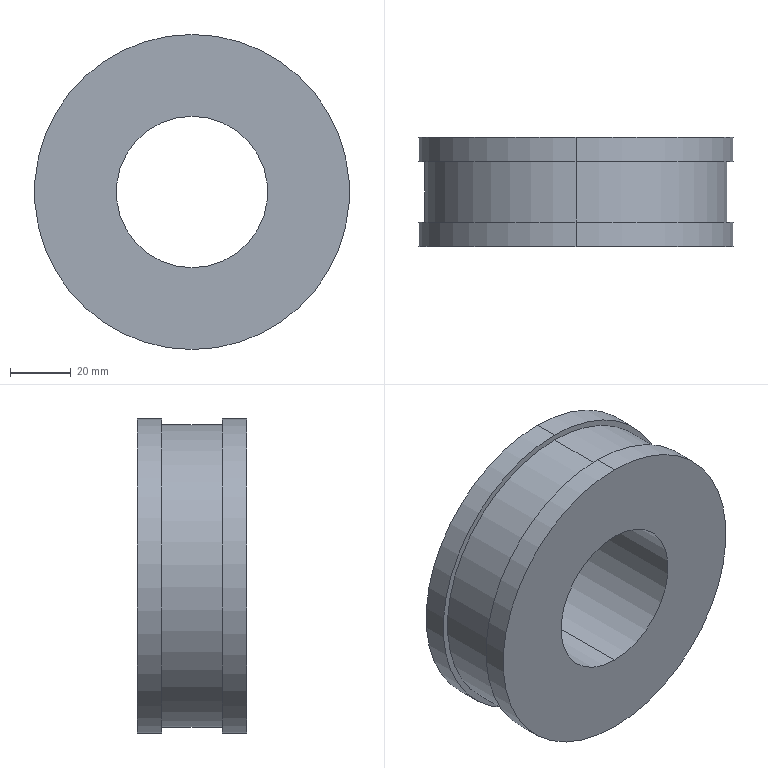Part | SolidWorks | features ICE 3, Extrusion 1 | 1 solid | 12 faces | box 104 x 36 x 104 mm | volume 222312 mm3 | cylinder 8 | plane 4 | commonest cylinder face diameters 104 x4 50 x2 100 x2
STEP:
#1=CARTESIAN_POINT('',(0.,28.,25.));
#2=VERTEX_POINT('',#1);
#3=CARTESIAN_POINT('',(0.,28.,-25.));
#4=VERTEX_POINT('',#3);
#5=CARTESIAN_POINT('',(0.,28.,0.));
#6=DIRECTION('',(0.,-1.,0.));
#7=DIRECTION('',(0.,0.,-1.));
#8=AXIS2_PLACEMENT_3D('',#5,#6,#7);
#9=CIRCLE('',#8,25.);
#10=EDGE_CURVE('',#2,#4,#9,.T.);
#11=ORIENTED_EDGE('',*,*,#10,.F.);
#12=CARTESIAN_POINT('',(0.,-8.,25.));
#13=VERTEX_POINT('',#12);
#14=CARTESIAN_POINT('',(0.,28.,25.));
#15=DIRECTION('',(0.,-1.,0.));
#16=VECTOR('',#15,1000.);
#17=LINE('',#14,#16);
#18=EDGE_CURVE('',#2,#13,#17,.T.);
#19=ORIENTED_EDGE('',*,*,#18,.T.);
#20=CARTESIAN_POINT('',(0.,-8.,-25.));
#21=VERTEX_POINT('',#20);
#22=CARTESIAN_POINT('',(0.,-8.,0.));
#23=DIRECTION('',(0.,-1.,0.));
#24=DIRECTION('',(0.,0.,-1.));
#25=AXIS2_PLACEMENT_3D('',#22,#23,#24);
#26=CIRCLE('',#25,25.);
#27=EDGE_CURVE('',#13,#21,#26,.T.);
#28=ORIENTED_EDGE('',*,*,#27,.T.);
#29=CARTESIAN_POINT('',(0.,28.,-25.));
#30=DIRECTION('',(0.,-1.,0.));
#31=VECTOR('',#30,1000.);
#32=LINE('',#29,#31);
#33=EDGE_CURVE('',#4,#21,#32,.T.);
#34=ORIENTED_EDGE('',*,*,#33,.F.);
#35=EDGE_LOOP('',(#11,#19,#28,#34));
#36=FACE_OUTER_BOUND('',#35,.T.);
#37=CARTESIAN_POINT('',(0.,28.,0.));
#38=DIRECTION('',(0.,-1.,0.));
#39=DIRECTION('',(0.,0.,-1.));
#40=AXIS2_PLACEMENT_3D('',#37,#38,#39);
#41=CYLINDRICAL_SURFACE('',#40,25.);
#42=ADVANCED_FACE('',(#36),#41,.F.);
#43=CARTESIAN_POINT('',(0.,-8.,-52.));
#44=VERTEX_POINT('',#43);
#45=CARTESIAN_POINT('',(0.,-8.,52.));
#46=VERTEX_POINT('',#45);
#47=CARTESIAN_POINT('',(0.,-8.,0.));
#48=DIRECTION('',(0.,-1.,0.));
#49=DIRECTION('',(0.,0.,-1.));
#50=AXIS2_PLACEMENT_3D('',#47,#48,#49);
#51=CIRCLE('',#50,52.);
#52=EDGE_CURVE('',#44,#46,#51,.T.);
#53=ORIENTED_EDGE('',*,*,#52,.F.);
#54=CARTESIAN_POINT('',(0.,0.,-52.));
#55=VERTEX_POINT('',#54);
#56=CARTESIAN_POINT('',(0.,-8.,-52.));
#57=DIRECTION('',(0.,1.,0.));
#58=VECTOR('',#57,1000.);
#59=LINE('',#56,#58);
#60=EDGE_CURVE('',#44,#55,#59,.T.);
#61=ORIENTED_EDGE('',*,*,#60,.T.);
#62=CARTESIAN_POINT('',(0.,0.,52.));
#63=VERTEX_POINT('',#62);
#64=CARTESIAN_POINT('',(0.,0.,0.));
#65=DIRECTION('',(0.,-1.,0.));
#66=DIRECTION('',(0.,0.,-1.));
#67=AXIS2_PLACEMENT_3D('',#64,#65,#66);
#68=CIRCLE('',#67,52.);
#69=EDGE_CURVE('',#55,#63,#68,.T.);
#70=ORIENTED_EDGE('',*,*,#69,.T.);
#71=CARTESIAN_POINT('',(0.,-8.,52.));
#72=DIRECTION('',(0.,1.,0.));
#73=VECTOR('',#72,1000.);
#74=LINE('',#71,#73);
#75=EDGE_CURVE('',#46,#63,#74,.T.);
#76=ORIENTED_EDGE('',*,*,#75,.F.);
#77=EDGE_LOOP('',(#53,#61,#70,#76));
#78=FACE_OUTER_BOUND('',#77,.T.);
#79=CARTESIAN_POINT('',(0.,-8.,0.));
#80=DIRECTION('',(0.,1.,0.));
#81=DIRECTION('',(0.,0.,1.));
#82=AXIS2_PLACEMENT_3D('',#79,#80,#81);
#83=CYLINDRICAL_SURFACE('',#82,52.);
#84=ADVANCED_FACE('',(#78),#83,.T.);
#85=CARTESIAN_POINT('',(0.,28.,52.));
#86=VERTEX_POINT('',#85);
#87=CARTESIAN_POINT('',(0.,28.,-52.));
#88=VERTEX_POINT('',#87);
#89=CARTESIAN_POINT('',(0.,28.,0.));
#90=DIRECTION('',(0.,1.,0.));
#91=DIRECTION('',(0.,0.,1.));
#92=AXIS2_PLACEMENT_3D('',#89,#90,#91);
#93=CIRCLE('',#92,52.);
#94=EDGE_CURVE('',#86,#88,#93,.T.);
#95=ORIENTED_EDGE('',*,*,#94,.F.);
#96=CARTESIAN_POINT('',(0.,20.,52.));
#97=VERTEX_POINT('',#96);
#98=CARTESIAN_POINT('',(0.,28.,52.));
#99=DIRECTION('',(0.,-1.,0.));
#100=VECTOR('',#99,1000.);
#101=LINE('',#98,#100);
#102=EDGE_CURVE('',#86,#97,#101,.T.);
#103=ORIENTED_EDGE('',*,*,#102,.T.);
#104=CARTESIAN_POINT('',(0.,20.,-52.));
#105=VERTEX_POINT('',#104);
#106=CARTESIAN_POINT('',(0.,20.,0.));
#107=DIRECTION('',(0.,1.,0.));
#108=DIRECTION('',(0.,0.,1.));
#109=AXIS2_PLACEMENT_3D('',#106,#107,#108);
#110=CIRCLE('',#109,52.);
#111=EDGE_CURVE('',#97,#105,#110,.T.);
#112=ORIENTED_EDGE('',*,*,#111,.T.);
#113=CARTESIAN_POINT('',(0.,28.,-52.));
#114=DIRECTION('',(0.,-1.,0.));
#115=VECTOR('',#114,1000.);
#116=LINE('',#113,#115);
#117=EDGE_CURVE('',#88,#105,#116,.T.);
#118=ORIENTED_EDGE('',*,*,#117,.F.);
#119=EDGE_LOOP('',(#95,#103,#112,#118));
#120=FACE_OUTER_BOUND('',#119,.T.);
#121=CARTESIAN_POINT('',(0.,28.,0.));
#122=DIRECTION('',(0.,-1.,0.));
#123=DIRECTION('',(0.,0.,-1.));
#124=AXIS2_PLACEMENT_3D('',#121,#122,#123);
#125=CYLINDRICAL_SURFACE('',#124,52.);
#126=ADVANCED_FACE('',(#120),#125,.T.);
#127=CARTESIAN_POINT('',(0.,20.,50.));
#128=VERTEX_POINT('',#127);
#129=CARTESIAN_POINT('',(0.,20.,-50.));
#130=VERTEX_POINT('',#129);
#131=CARTESIAN_POINT('',(0.,20.,0.));
#132=DIRECTION('',(0.,1.,0.));
#133=DIRECTION('',(0.,0.,1.));
#134=AXIS2_PLACEMENT_3D('',#131,#132,#133);
#135=CIRCLE('',#134,50.);
#136=EDGE_CURVE('',#128,#130,#135,.T.);
#137=ORIENTED_EDGE('',*,*,#136,.F.);
#138=CARTESIAN_POINT('',(0.,0.,50.));
#139=VERTEX_POINT('',#138);
#140=CARTESIAN_POINT('',(0.,20.,50.));
#141=DIRECTION('',(0.,-1.,0.));
#142=VECTOR('',#141,1000.);
#143=LINE('',#140,#142);
#144=EDGE_CURVE('',#128,#139,#143,.T.);
#145=ORIENTED_EDGE('',*,*,#144,.T.);
#146=CARTESIAN_POINT('',(0.,0.,-50.));
#147=VERTEX_POINT('',#146);
#148=CARTESIAN_POINT('',(0.,0.,0.));
#149=DIRECTION('',(0.,-1.,0.));
#150=DIRECTION('',(0.,0.,-1.));
#151=AXIS2_PLACEMENT_3D('',#148,#149,#150);
#152=CIRCLE('',#151,50.);
#153=EDGE_CURVE('',#147,#139,#152,.T.);
#154=ORIENTED_EDGE('',*,*,#153,.F.);
#155=CARTESIAN_POINT('',(0.,20.,-50.));
#156=DIRECTION('',(0.,-1.,0.));
#157=VECTOR('',#156,1000.);
#158=LINE('',#155,#157);
#159=EDGE_CURVE('',#130,#147,#158,.T.);
#160=ORIENTED_EDGE('',*,*,#159,.F.);
#161=EDGE_LOOP('',(#137,#145,#154,#160));
#162=FACE_OUTER_BOUND('',#161,.T.);
#163=CARTESIAN_POINT('',(0.,20.,0.));
#164=DIRECTION('',(0.,-1.,0.));
#165=DIRECTION('',(0.,0.,-1.));
#166=AXIS2_PLACEMENT_3D('',#163,#164,#165);
#167=CYLINDRICAL_SURFACE('',#166,50.);
#168=ADVANCED_FACE('',(#162),#167,.T.);
#169=ORIENTED_EDGE('',*,*,#144,.F.);
#170=CARTESIAN_POINT('',(0.,20.,0.));
#171=DIRECTION('',(0.,1.,0.));
#172=DIRECTION('',(0.,0.,1.));
#173=AXIS2_PLACEMENT_3D('',#170,#171,#172);
#174=CIRCLE('',#173,50.);
#175=EDGE_CURVE('',#130,#128,#174,.T.);
#176=ORIENTED_EDGE('',*,*,#175,.F.);
#177=ORIENTED_EDGE('',*,*,#159,.T.);
#178=CARTESIAN_POINT('',(0.,0.,0.));
#179=DIRECTION('',(0.,-1.,0.));
#180=DIRECTION('',(0.,0.,-1.));
#181=AXIS2_PLACEMENT_3D('',#178,#179,#180);
#182=CIRCLE('',#181,50.);
#183=EDGE_CURVE('',#139,#147,#182,.T.);
#184=ORIENTED_EDGE('',*,*,#183,.F.);
#185=EDGE_LOOP('',(#169,#176,#177,#184));
#186=FACE_OUTER_BOUND('',#185,.T.);
#187=CARTESIAN_POINT('',(0.,20.,0.));
#188=DIRECTION('',(0.,-1.,0.));
#189=DIRECTION('',(0.,0.,-1.));
#190=AXIS2_PLACEMENT_3D('',#187,#188,#189);
#191=CYLINDRICAL_SURFACE('',#190,50.);
#192=ADVANCED_FACE('',(#186),#191,.T.);
#193=CARTESIAN_POINT('',(0.,20.,0.));
#194=DIRECTION('',(0.,1.,0.));
#195=DIRECTION('',(0.,0.,1.));
#196=AXIS2_PLACEMENT_3D('',#193,#194,#195);
#197=CIRCLE('',#196,52.);
#198=EDGE_CURVE('',#105,#97,#197,.T.);
#199=ORIENTED_EDGE('',*,*,#198,.F.);
#200=ORIENTED_EDGE('',*,*,#111,.F.);
#201=EDGE_LOOP('',(#199,#200));
#202=FACE_OUTER_BOUND('',#201,.T.);
#203=ORIENTED_EDGE('',*,*,#175,.T.);
#204=ORIENTED_EDGE('',*,*,#136,.T.);
#205=EDGE_LOOP('',(#203,#204));
#206=FACE_BOUND('',#205,.T.);
#207=CARTESIAN_POINT('',(0.,20.,0.));
#208=DIRECTION('',(0.,1.,0.));
#209=DIRECTION('',(0.,0.,1.));
#210=AXIS2_PLACEMENT_3D('',#207,#208,#209);
#211=PLANE('',#210);
#212=ADVANCED_FACE('',(#202,#206),#211,.F.);
#213=ORIENTED_EDGE('',*,*,#102,.F.);
#214=CARTESIAN_POINT('',(0.,28.,0.));
#215=DIRECTION('',(0.,1.,0.));
#216=DIRECTION('',(0.,0.,1.));
#217=AXIS2_PLACEMENT_3D('',#214,#215,#216);
#218=CIRCLE('',#217,52.);
#219=EDGE_CURVE('',#88,#86,#218,.T.);
#220=ORIENTED_EDGE('',*,*,#219,.F.);
#221=ORIENTED_EDGE('',*,*,#117,.T.);
#222=ORIENTED_EDGE('',*,*,#198,.T.);
#223=EDGE_LOOP('',(#213,#220,#221,#222));
#224=FACE_OUTER_BOUND('',#223,.T.);
#225=CARTESIAN_POINT('',(0.,28.,0.));
#226=DIRECTION('',(0.,-1.,0.));
#227=DIRECTION('',(0.,0.,-1.));
#228=AXIS2_PLACEMENT_3D('',#225,#226,#227);
#229=CYLINDRICAL_SURFACE('',#228,52.);
#230=ADVANCED_FACE('',(#224),#229,.T.);
#231=CARTESIAN_POINT('',(0.,28.,0.));
#232=DIRECTION('',(0.,-1.,0.));
#233=DIRECTION('',(0.,0.,-1.));
#234=AXIS2_PLACEMENT_3D('',#231,#232,#233);
#235=CIRCLE('',#234,25.);
#236=EDGE_CURVE('',#4,#2,#235,.T.);
#237=ORIENTED_EDGE('',*,*,#236,.T.);
#238=ORIENTED_EDGE('',*,*,#10,.T.);
#239=EDGE_LOOP('',(#237,#238));
#240=FACE_BOUND('',#239,.T.);
#241=ORIENTED_EDGE('',*,*,#219,.T.);
#242=ORIENTED_EDGE('',*,*,#94,.T.);
#243=EDGE_LOOP('',(#241,#242));
#244=FACE_OUTER_BOUND('',#243,.T.);
#245=CARTESIAN_POINT('',(0.,28.,0.));
#246=DIRECTION('',(0.,1.,0.));
#247=DIRECTION('',(0.,0.,1.));
#248=AXIS2_PLACEMENT_3D('',#245,#246,#247);
#249=PLANE('',#248);
#250=ADVANCED_FACE('',(#240,#244),#249,.T.);
#251=CARTESIAN_POINT('',(0.,0.,0.));
#252=DIRECTION('',(0.,-1.,0.));
#253=DIRECTION('',(0.,0.,-1.));
#254=AXIS2_PLACEMENT_3D('',#251,#252,#253);
#255=CIRCLE('',#254,52.);
#256=EDGE_CURVE('',#63,#55,#255,.T.);
#257=ORIENTED_EDGE('',*,*,#256,.F.);
#258=ORIENTED_EDGE('',*,*,#69,.F.);
#259=EDGE_LOOP('',(#257,#258));
#260=FACE_OUTER_BOUND('',#259,.T.);
#261=ORIENTED_EDGE('',*,*,#153,.T.);
#262=ORIENTED_EDGE('',*,*,#183,.T.);
#263=EDGE_LOOP('',(#261,#262));
#264=FACE_BOUND('',#263,.T.);
#265=CARTESIAN_POINT('',(0.,0.,0.));
#266=DIRECTION('',(0.,-1.,0.));
#267=DIRECTION('',(0.,0.,-1.));
#268=AXIS2_PLACEMENT_3D('',#265,#266,#267);
#269=PLANE('',#268);
#270=ADVANCED_FACE('',(#260,#264),#269,.F.);
#271=ORIENTED_EDGE('',*,*,#60,.F.);
#272=CARTESIAN_POINT('',(0.,-8.,0.));
#273=DIRECTION('',(0.,-1.,0.));
#274=DIRECTION('',(0.,0.,-1.));
#275=AXIS2_PLACEMENT_3D('',#272,#273,#274);
#276=CIRCLE('',#275,52.);
#277=EDGE_CURVE('',#46,#44,#276,.T.);
#278=ORIENTED_EDGE('',*,*,#277,.F.);
#279=ORIENTED_EDGE('',*,*,#75,.T.);
#280=ORIENTED_EDGE('',*,*,#256,.T.);
#281=EDGE_LOOP('',(#271,#278,#279,#280));
#282=FACE_OUTER_BOUND('',#281,.T.);
#283=CARTESIAN_POINT('',(0.,-8.,0.));
#284=DIRECTION('',(0.,1.,0.));
#285=DIRECTION('',(0.,0.,1.));
#286=AXIS2_PLACEMENT_3D('',#283,#284,#285);
#287=CYLINDRICAL_SURFACE('',#286,52.);
#288=ADVANCED_FACE('',(#282),#287,.T.);
#289=CARTESIAN_POINT('',(0.,-8.,0.));
#290=DIRECTION('',(0.,-1.,0.));
#291=DIRECTION('',(0.,0.,-1.));
#292=AXIS2_PLACEMENT_3D('',#289,#290,#291);
#293=CIRCLE('',#292,25.);
#294=EDGE_CURVE('',#21,#13,#293,.T.);
#295=ORIENTED_EDGE('',*,*,#294,.F.);
#296=ORIENTED_EDGE('',*,*,#27,.F.);
#297=EDGE_LOOP('',(#295,#296));
#298=FACE_BOUND('',#297,.T.);
#299=ORIENTED_EDGE('',*,*,#277,.T.);
#300=ORIENTED_EDGE('',*,*,#52,.T.);
#301=EDGE_LOOP('',(#299,#300));
#302=FACE_OUTER_BOUND('',#301,.T.);
#303=CARTESIAN_POINT('',(0.,-8.,0.));
#304=DIRECTION('',(0.,-1.,0.));
#305=DIRECTION('',(0.,0.,-1.));
#306=AXIS2_PLACEMENT_3D('',#303,#304,#305);
#307=PLANE('',#306);
#308=ADVANCED_FACE('',(#298,#302),#307,.T.);
#309=ORIENTED_EDGE('',*,*,#18,.F.);
#310=ORIENTED_EDGE('',*,*,#236,.F.);
#311=ORIENTED_EDGE('',*,*,#33,.T.);
#312=ORIENTED_EDGE('',*,*,#294,.T.);
#313=EDGE_LOOP('',(#309,#310,#311,#312));
#314=FACE_OUTER_BOUND('',#313,.T.);
#315=CARTESIAN_POINT('',(0.,28.,0.));
#316=DIRECTION('',(0.,-1.,0.));
#317=DIRECTION('',(0.,0.,-1.));
#318=AXIS2_PLACEMENT_3D('',#315,#316,#317);
#319=CYLINDRICAL_SURFACE('',#318,25.);
#320=ADVANCED_FACE('',(#314),#319,.F.);
#321=CLOSED_SHELL('',(#42,#84,#126,#168,#192,#212,#230,#250,#270,#288,#308,#320));
#322=MANIFOLD_SOLID_BREP('',#321);
#323=CARTESIAN_POINT('',(0.,0.,0.));
#324=DIRECTION('',(0.,0.,1.));
#325=DIRECTION('',(1.,0.,0.));
#326=AXIS2_PLACEMENT_3D('',#323,#324,#325);
#327=(LENGTH_UNIT()NAMED_UNIT(*)SI_UNIT(.MILLI.,.METRE.));
#328=UNCERTAINTY_MEASURE_WITH_UNIT(LENGTH_MEASURE(0.00001),#327,'','');
#329=(NAMED_UNIT(*)PLANE_ANGLE_UNIT()SI_UNIT($,.RADIAN.));
#330=(NAMED_UNIT(*)SI_UNIT($,.STERADIAN.)SOLID_ANGLE_UNIT());
#331=(GEOMETRIC_REPRESENTATION_CONTEXT(3)GLOBAL_UNCERTAINTY_ASSIGNED_CONTEXT((#328))GLOBAL_UNIT_ASSIGNED_CONTEXT((#327,#329,#330))REPRESENTATION_CONTEXT('',''));
#332=ADVANCED_BREP_SHAPE_REPRESENTATION('',(#322,#326),#331);